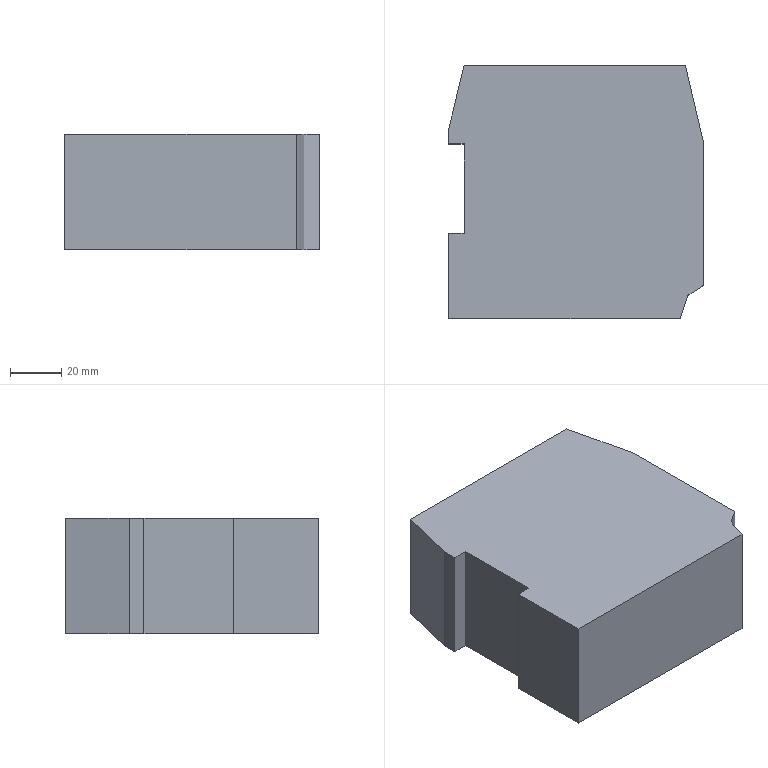Part | STEP file | EMC filter FIL-1S-1-10A-230AC-UT   1292320 | 1 solid | 14 faces | box 99.5 x 99 x 45 mm | volume 422145 mm3 | plane 14
STEP:
#1=CARTESIAN_POINT('',(0.,0.,0.));
#2=DIRECTION('',(0.,0.,1.));
#3=DIRECTION('',(1.,0.,0.));
#4=AXIS2_PLACEMENT_3D('',#1,#2,#3);
#5=CARTESIAN_POINT('',(49.75,18.24,0.));
#6=VERTEX_POINT('',#5);
#7=CARTESIAN_POINT('',(42.75,48.24,0.));
#8=VERTEX_POINT('',#7);
#9=CARTESIAN_POINT('',(42.75,48.24,0.));
#10=DIRECTION('',(-0.2272,0.9738,0.));
#11=VECTOR('',#10,1.);
#12=LINE('',#9,#11);
#13=CARTESIAN_POINT('',(42.75,48.24,45.));
#14=DIRECTION('',(-0.9738,-0.2272,0.));
#15=DIRECTION('',(0.2272,-0.9738,0.));
#16=AXIS2_PLACEMENT_3D('',#13,#14,#15);
#17=PLANE('',#16);
#18=CARTESIAN_POINT('',(0.,-45.));
#19=DIRECTION('',(-1.,0.));
#20=VECTOR('',#19,1.);
#21=LINE('',#18,#20);
#22=(GEOMETRIC_REPRESENTATION_CONTEXT(2)PARAMETRIC_REPRESENTATION_CONTEXT()REPRESENTATION_CONTEXT('',''));
#23=DEFINITIONAL_REPRESENTATION('',(#21),#22);
#24=PCURVE('',#17,#23);
#25=CARTESIAN_POINT('',(0.,0.,0.));
#26=DIRECTION('',(0.,0.,1.));
#27=DIRECTION('',(1.,0.,0.));
#28=AXIS2_PLACEMENT_3D('',#25,#26,#27);
#29=PLANE('',#28);
#30=CARTESIAN_POINT('',(42.75,48.24));
#31=DIRECTION('',(-0.2272,0.9738));
#32=VECTOR('',#31,1.);
#33=LINE('',#30,#32);
#34=(GEOMETRIC_REPRESENTATION_CONTEXT(2)PARAMETRIC_REPRESENTATION_CONTEXT()REPRESENTATION_CONTEXT('',''));
#35=DEFINITIONAL_REPRESENTATION('',(#33),#34);
#36=PCURVE('',#29,#35);
#37=SURFACE_CURVE('',#12,(#24,#36),.PCURVE_S1.);
#38=EDGE_CURVE('',#6,#8,#37,.T.);
#39=ORIENTED_EDGE('',*,*,#38,.T.);
#40=CARTESIAN_POINT('',(42.75,48.24,45.));
#41=VERTEX_POINT('',#40);
#42=CARTESIAN_POINT('',(42.75,48.24,45.));
#43=DIRECTION('',(0.,0.,-1.));
#44=VECTOR('',#43,1.);
#45=LINE('',#42,#44);
#46=CARTESIAN_POINT('',(0.,0.));
#47=DIRECTION('',(0.,-1.));
#48=VECTOR('',#47,1.);
#49=LINE('',#46,#48);
#50=(GEOMETRIC_REPRESENTATION_CONTEXT(2)PARAMETRIC_REPRESENTATION_CONTEXT()REPRESENTATION_CONTEXT('',''));
#51=DEFINITIONAL_REPRESENTATION('',(#49),#50);
#52=PCURVE('',#17,#51);
#53=CARTESIAN_POINT('',(-43.75,48.24,45.));
#54=DIRECTION('',(0.,-1.,0.));
#55=DIRECTION('',(0.,0.,-1.));
#56=AXIS2_PLACEMENT_3D('',#53,#54,#55);
#57=PLANE('',#56);
#58=CARTESIAN_POINT('',(0.,86.5));
#59=DIRECTION('',(1.,0.));
#60=VECTOR('',#59,1.);
#61=LINE('',#58,#60);
#62=(GEOMETRIC_REPRESENTATION_CONTEXT(2)PARAMETRIC_REPRESENTATION_CONTEXT()REPRESENTATION_CONTEXT('',''));
#63=DEFINITIONAL_REPRESENTATION('',(#61),#62);
#64=PCURVE('',#57,#63);
#65=SURFACE_CURVE('',#45,(#52,#64),.PCURVE_S1.);
#66=EDGE_CURVE('',#41,#8,#65,.T.);
#67=ORIENTED_EDGE('',*,*,#66,.F.);
#68=CARTESIAN_POINT('',(49.75,18.24,45.));
#69=VERTEX_POINT('',#68);
#70=CARTESIAN_POINT('',(42.75,48.24,45.));
#71=DIRECTION('',(-0.2272,0.9738,0.));
#72=VECTOR('',#71,1.);
#73=LINE('',#70,#72);
#74=CARTESIAN_POINT('',(0.,0.));
#75=DIRECTION('',(-1.,0.));
#76=VECTOR('',#75,1.);
#77=LINE('',#74,#76);
#78=(GEOMETRIC_REPRESENTATION_CONTEXT(2)PARAMETRIC_REPRESENTATION_CONTEXT()REPRESENTATION_CONTEXT('',''));
#79=DEFINITIONAL_REPRESENTATION('',(#77),#78);
#80=PCURVE('',#17,#79);
#81=CARTESIAN_POINT('',(0.,0.,45.));
#82=DIRECTION('',(0.,0.,1.));
#83=DIRECTION('',(1.,0.,0.));
#84=AXIS2_PLACEMENT_3D('',#81,#82,#83);
#85=PLANE('',#84);
#86=CARTESIAN_POINT('',(42.75,48.24));
#87=DIRECTION('',(-0.2272,0.9738));
#88=VECTOR('',#87,1.);
#89=LINE('',#86,#88);
#90=(GEOMETRIC_REPRESENTATION_CONTEXT(2)PARAMETRIC_REPRESENTATION_CONTEXT()REPRESENTATION_CONTEXT('',''));
#91=DEFINITIONAL_REPRESENTATION('',(#89),#90);
#92=PCURVE('',#85,#91);
#93=SURFACE_CURVE('',#73,(#80,#92),.PCURVE_S1.);
#94=EDGE_CURVE('',#69,#41,#93,.T.);
#95=ORIENTED_EDGE('',*,*,#94,.F.);
#96=CARTESIAN_POINT('',(49.75,18.24,45.));
#97=DIRECTION('',(0.,0.,-1.));
#98=VECTOR('',#97,1.);
#99=LINE('',#96,#98);
#100=CARTESIAN_POINT('',(30.806,0.));
#101=DIRECTION('',(0.,-1.));
#102=VECTOR('',#101,1.);
#103=LINE('',#100,#102);
#104=(GEOMETRIC_REPRESENTATION_CONTEXT(2)PARAMETRIC_REPRESENTATION_CONTEXT()REPRESENTATION_CONTEXT('',''));
#105=DEFINITIONAL_REPRESENTATION('',(#103),#104);
#106=PCURVE('',#17,#105);
#107=CARTESIAN_POINT('',(49.75,18.24,45.));
#108=DIRECTION('',(-1.,0.,0.));
#109=DIRECTION('',(0.,-1.,0.));
#110=AXIS2_PLACEMENT_3D('',#107,#108,#109);
#111=PLANE('',#110);
#112=CARTESIAN_POINT('',(0.,0.));
#113=DIRECTION('',(0.,-1.));
#114=VECTOR('',#113,1.);
#115=LINE('',#112,#114);
#116=(GEOMETRIC_REPRESENTATION_CONTEXT(2)PARAMETRIC_REPRESENTATION_CONTEXT()REPRESENTATION_CONTEXT('',''));
#117=DEFINITIONAL_REPRESENTATION('',(#115),#116);
#118=PCURVE('',#111,#117);
#119=SURFACE_CURVE('',#99,(#106,#118),.PCURVE_S1.);
#120=EDGE_CURVE('',#69,#6,#119,.T.);
#121=ORIENTED_EDGE('',*,*,#120,.T.);
#122=EDGE_LOOP('',(#39,#67,#95,#121));
#123=FACE_BOUND('',#122,.T.);
#124=ADVANCED_FACE('',(#123),#17,.F.);
#125=CARTESIAN_POINT('',(-43.75,48.24,0.));
#126=VERTEX_POINT('',#125);
#127=CARTESIAN_POINT('',(-43.75,48.24,0.));
#128=DIRECTION('',(-1.,0.,0.));
#129=VECTOR('',#128,1.);
#130=LINE('',#127,#129);
#131=CARTESIAN_POINT('',(45.,0.));
#132=DIRECTION('',(0.,-1.));
#133=VECTOR('',#132,1.);
#134=LINE('',#131,#133);
#135=(GEOMETRIC_REPRESENTATION_CONTEXT(2)PARAMETRIC_REPRESENTATION_CONTEXT()REPRESENTATION_CONTEXT('',''));
#136=DEFINITIONAL_REPRESENTATION('',(#134),#135);
#137=PCURVE('',#57,#136);
#138=CARTESIAN_POINT('',(-43.75,48.24));
#139=DIRECTION('',(-1.,0.));
#140=VECTOR('',#139,1.);
#141=LINE('',#138,#140);
#142=(GEOMETRIC_REPRESENTATION_CONTEXT(2)PARAMETRIC_REPRESENTATION_CONTEXT()REPRESENTATION_CONTEXT('',''));
#143=DEFINITIONAL_REPRESENTATION('',(#141),#142);
#144=PCURVE('',#29,#143);
#145=SURFACE_CURVE('',#130,(#137,#144),.PCURVE_S1.);
#146=EDGE_CURVE('',#8,#126,#145,.T.);
#147=ORIENTED_EDGE('',*,*,#146,.T.);
#148=CARTESIAN_POINT('',(-43.75,48.24,45.));
#149=VERTEX_POINT('',#148);
#150=CARTESIAN_POINT('',(-43.75,48.24,45.));
#151=DIRECTION('',(0.,0.,-1.));
#152=VECTOR('',#151,1.);
#153=LINE('',#150,#152);
#154=CARTESIAN_POINT('',(0.,0.));
#155=DIRECTION('',(1.,0.));
#156=VECTOR('',#155,1.);
#157=LINE('',#154,#156);
#158=(GEOMETRIC_REPRESENTATION_CONTEXT(2)PARAMETRIC_REPRESENTATION_CONTEXT()REPRESENTATION_CONTEXT('',''));
#159=DEFINITIONAL_REPRESENTATION('',(#157),#158);
#160=PCURVE('',#57,#159);
#161=CARTESIAN_POINT('',(-49.75,23.24,45.));
#162=DIRECTION('',(0.9724,-0.2334,0.));
#163=DIRECTION('',(0.2334,0.9724,0.));
#164=AXIS2_PLACEMENT_3D('',#161,#162,#163);
#165=PLANE('',#164);
#166=CARTESIAN_POINT('',(25.71,0.));
#167=DIRECTION('',(0.,-1.));
#168=VECTOR('',#167,1.);
#169=LINE('',#166,#168);
#170=(GEOMETRIC_REPRESENTATION_CONTEXT(2)PARAMETRIC_REPRESENTATION_CONTEXT()REPRESENTATION_CONTEXT('',''));
#171=DEFINITIONAL_REPRESENTATION('',(#169),#170);
#172=PCURVE('',#165,#171);
#173=SURFACE_CURVE('',#153,(#160,#172),.PCURVE_S1.);
#174=EDGE_CURVE('',#149,#126,#173,.T.);
#175=ORIENTED_EDGE('',*,*,#174,.F.);
#176=CARTESIAN_POINT('',(-43.75,48.24,45.));
#177=DIRECTION('',(-1.,0.,0.));
#178=VECTOR('',#177,1.);
#179=LINE('',#176,#178);
#180=CARTESIAN_POINT('',(0.,0.));
#181=DIRECTION('',(0.,-1.));
#182=VECTOR('',#181,1.);
#183=LINE('',#180,#182);
#184=(GEOMETRIC_REPRESENTATION_CONTEXT(2)PARAMETRIC_REPRESENTATION_CONTEXT()REPRESENTATION_CONTEXT('',''));
#185=DEFINITIONAL_REPRESENTATION('',(#183),#184);
#186=PCURVE('',#57,#185);
#187=CARTESIAN_POINT('',(-43.75,48.24));
#188=DIRECTION('',(-1.,0.));
#189=VECTOR('',#188,1.);
#190=LINE('',#187,#189);
#191=(GEOMETRIC_REPRESENTATION_CONTEXT(2)PARAMETRIC_REPRESENTATION_CONTEXT()REPRESENTATION_CONTEXT('',''));
#192=DEFINITIONAL_REPRESENTATION('',(#190),#191);
#193=PCURVE('',#85,#192);
#194=SURFACE_CURVE('',#179,(#186,#193),.PCURVE_S1.);
#195=EDGE_CURVE('',#41,#149,#194,.T.);
#196=ORIENTED_EDGE('',*,*,#195,.F.);
#197=ORIENTED_EDGE('',*,*,#66,.T.);
#198=EDGE_LOOP('',(#147,#175,#196,#197));
#199=FACE_BOUND('',#198,.T.);
#200=ADVANCED_FACE('',(#199),#57,.F.);
#201=CARTESIAN_POINT('',(-49.75,23.24,0.));
#202=VERTEX_POINT('',#201);
#203=CARTESIAN_POINT('',(-49.75,23.24,0.));
#204=DIRECTION('',(-0.2334,-0.9724,0.));
#205=VECTOR('',#204,1.);
#206=LINE('',#203,#205);
#207=CARTESIAN_POINT('',(0.,-45.));
#208=DIRECTION('',(-1.,0.));
#209=VECTOR('',#208,1.);
#210=LINE('',#207,#209);
#211=(GEOMETRIC_REPRESENTATION_CONTEXT(2)PARAMETRIC_REPRESENTATION_CONTEXT()REPRESENTATION_CONTEXT('',''));
#212=DEFINITIONAL_REPRESENTATION('',(#210),#211);
#213=PCURVE('',#165,#212);
#214=CARTESIAN_POINT('',(-49.75,23.24));
#215=DIRECTION('',(-0.2334,-0.9724));
#216=VECTOR('',#215,1.);
#217=LINE('',#214,#216);
#218=(GEOMETRIC_REPRESENTATION_CONTEXT(2)PARAMETRIC_REPRESENTATION_CONTEXT()REPRESENTATION_CONTEXT('',''));
#219=DEFINITIONAL_REPRESENTATION('',(#217),#218);
#220=PCURVE('',#29,#219);
#221=SURFACE_CURVE('',#206,(#213,#220),.PCURVE_S1.);
#222=EDGE_CURVE('',#126,#202,#221,.T.);
#223=ORIENTED_EDGE('',*,*,#222,.T.);
#224=CARTESIAN_POINT('',(-49.75,23.24,45.));
#225=VERTEX_POINT('',#224);
#226=CARTESIAN_POINT('',(-49.75,23.24,45.));
#227=DIRECTION('',(0.,0.,-1.));
#228=VECTOR('',#227,1.);
#229=LINE('',#226,#228);
#230=CARTESIAN_POINT('',(0.,0.));
#231=DIRECTION('',(0.,-1.));
#232=VECTOR('',#231,1.);
#233=LINE('',#230,#232);
#234=(GEOMETRIC_REPRESENTATION_CONTEXT(2)PARAMETRIC_REPRESENTATION_CONTEXT()REPRESENTATION_CONTEXT('',''));
#235=DEFINITIONAL_REPRESENTATION('',(#233),#234);
#236=PCURVE('',#165,#235);
#237=CARTESIAN_POINT('',(-49.75,23.24,45.));
#238=DIRECTION('',(1.,0.,0.));
#239=DIRECTION('',(0.,0.,-1.));
#240=AXIS2_PLACEMENT_3D('',#237,#238,#239);
#241=PLANE('',#240);
#242=CARTESIAN_POINT('',(0.,0.));
#243=DIRECTION('',(1.,0.));
#244=VECTOR('',#243,1.);
#245=LINE('',#242,#244);
#246=(GEOMETRIC_REPRESENTATION_CONTEXT(2)PARAMETRIC_REPRESENTATION_CONTEXT()REPRESENTATION_CONTEXT('',''));
#247=DEFINITIONAL_REPRESENTATION('',(#245),#246);
#248=PCURVE('',#241,#247);
#249=SURFACE_CURVE('',#229,(#236,#248),.PCURVE_S1.);
#250=EDGE_CURVE('',#225,#202,#249,.T.);
#251=ORIENTED_EDGE('',*,*,#250,.F.);
#252=CARTESIAN_POINT('',(-49.75,23.24,45.));
#253=DIRECTION('',(-0.2334,-0.9724,0.));
#254=VECTOR('',#253,1.);
#255=LINE('',#252,#254);
#256=CARTESIAN_POINT('',(0.,0.));
#257=DIRECTION('',(-1.,0.));
#258=VECTOR('',#257,1.);
#259=LINE('',#256,#258);
#260=(GEOMETRIC_REPRESENTATION_CONTEXT(2)PARAMETRIC_REPRESENTATION_CONTEXT()REPRESENTATION_CONTEXT('',''));
#261=DEFINITIONAL_REPRESENTATION('',(#259),#260);
#262=PCURVE('',#165,#261);
#263=CARTESIAN_POINT('',(-49.75,23.24));
#264=DIRECTION('',(-0.2334,-0.9724));
#265=VECTOR('',#264,1.);
#266=LINE('',#263,#265);
#267=(GEOMETRIC_REPRESENTATION_CONTEXT(2)PARAMETRIC_REPRESENTATION_CONTEXT()REPRESENTATION_CONTEXT('',''));
#268=DEFINITIONAL_REPRESENTATION('',(#266),#267);
#269=PCURVE('',#85,#268);
#270=SURFACE_CURVE('',#255,(#262,#269),.PCURVE_S1.);
#271=EDGE_CURVE('',#149,#225,#270,.T.);
#272=ORIENTED_EDGE('',*,*,#271,.F.);
#273=ORIENTED_EDGE('',*,*,#174,.T.);
#274=EDGE_LOOP('',(#223,#251,#272,#273));
#275=FACE_BOUND('',#274,.T.);
#276=ADVANCED_FACE('',(#275),#165,.F.);
#277=CARTESIAN_POINT('',(-49.75,17.5,0.));
#278=VERTEX_POINT('',#277);
#279=CARTESIAN_POINT('',(-49.75,23.24,0.));
#280=DIRECTION('',(0.,-1.,0.));
#281=VECTOR('',#280,1.);
#282=LINE('',#279,#281);
#283=CARTESIAN_POINT('',(45.,0.));
#284=DIRECTION('',(0.,-1.));
#285=VECTOR('',#284,1.);
#286=LINE('',#283,#285);
#287=(GEOMETRIC_REPRESENTATION_CONTEXT(2)PARAMETRIC_REPRESENTATION_CONTEXT()REPRESENTATION_CONTEXT('',''));
#288=DEFINITIONAL_REPRESENTATION('',(#286),#287);
#289=PCURVE('',#241,#288);
#290=CARTESIAN_POINT('',(-49.75,23.24));
#291=DIRECTION('',(0.,-1.));
#292=VECTOR('',#291,1.);
#293=LINE('',#290,#292);
#294=(GEOMETRIC_REPRESENTATION_CONTEXT(2)PARAMETRIC_REPRESENTATION_CONTEXT()REPRESENTATION_CONTEXT('',''));
#295=DEFINITIONAL_REPRESENTATION('',(#293),#294);
#296=PCURVE('',#29,#295);
#297=SURFACE_CURVE('',#282,(#289,#296),.PCURVE_S1.);
#298=EDGE_CURVE('',#202,#278,#297,.T.);
#299=ORIENTED_EDGE('',*,*,#298,.T.);
#300=CARTESIAN_POINT('',(-49.75,17.5,45.));
#301=VERTEX_POINT('',#300);
#302=CARTESIAN_POINT('',(-49.75,17.5,45.));
#303=DIRECTION('',(0.,0.,-1.));
#304=VECTOR('',#303,1.);
#305=LINE('',#302,#304);
#306=CARTESIAN_POINT('',(0.,-5.74));
#307=DIRECTION('',(1.,0.));
#308=VECTOR('',#307,1.);
#309=LINE('',#306,#308);
#310=(GEOMETRIC_REPRESENTATION_CONTEXT(2)PARAMETRIC_REPRESENTATION_CONTEXT()REPRESENTATION_CONTEXT('',''));
#311=DEFINITIONAL_REPRESENTATION('',(#309),#310);
#312=PCURVE('',#241,#311);
#313=CARTESIAN_POINT('',(-49.75,17.5,45.));
#314=DIRECTION('',(0.,1.,0.));
#315=DIRECTION('',(0.,0.,1.));
#316=AXIS2_PLACEMENT_3D('',#313,#314,#315);
#317=PLANE('',#316);
#318=CARTESIAN_POINT('',(0.,0.));
#319=DIRECTION('',(-1.,0.));
#320=VECTOR('',#319,1.);
#321=LINE('',#318,#320);
#322=(GEOMETRIC_REPRESENTATION_CONTEXT(2)PARAMETRIC_REPRESENTATION_CONTEXT()REPRESENTATION_CONTEXT('',''));
#323=DEFINITIONAL_REPRESENTATION('',(#321),#322);
#324=PCURVE('',#317,#323);
#325=SURFACE_CURVE('',#305,(#312,#324),.PCURVE_S1.);
#326=EDGE_CURVE('',#301,#278,#325,.T.);
#327=ORIENTED_EDGE('',*,*,#326,.F.);
#328=CARTESIAN_POINT('',(-49.75,23.24,45.));
#329=DIRECTION('',(0.,-1.,0.));
#330=VECTOR('',#329,1.);
#331=LINE('',#328,#330);
#332=CARTESIAN_POINT('',(0.,0.));
#333=DIRECTION('',(0.,-1.));
#334=VECTOR('',#333,1.);
#335=LINE('',#332,#334);
#336=(GEOMETRIC_REPRESENTATION_CONTEXT(2)PARAMETRIC_REPRESENTATION_CONTEXT()REPRESENTATION_CONTEXT('',''));
#337=DEFINITIONAL_REPRESENTATION('',(#335),#336);
#338=PCURVE('',#241,#337);
#339=CARTESIAN_POINT('',(-49.75,23.24));
#340=DIRECTION('',(0.,-1.));
#341=VECTOR('',#340,1.);
#342=LINE('',#339,#341);
#343=(GEOMETRIC_REPRESENTATION_CONTEXT(2)PARAMETRIC_REPRESENTATION_CONTEXT()REPRESENTATION_CONTEXT('',''));
#344=DEFINITIONAL_REPRESENTATION('',(#342),#343);
#345=PCURVE('',#85,#344);
#346=SURFACE_CURVE('',#331,(#338,#345),.PCURVE_S1.);
#347=EDGE_CURVE('',#225,#301,#346,.T.);
#348=ORIENTED_EDGE('',*,*,#347,.F.);
#349=ORIENTED_EDGE('',*,*,#250,.T.);
#350=EDGE_LOOP('',(#299,#327,#348,#349));
#351=FACE_BOUND('',#350,.T.);
#352=ADVANCED_FACE('',(#351),#241,.F.);
#353=CARTESIAN_POINT('',(-43.75,17.5,0.));
#354=VERTEX_POINT('',#353);
#355=CARTESIAN_POINT('',(-49.75,17.5,0.));
#356=DIRECTION('',(1.,0.,0.));
#357=VECTOR('',#356,1.);
#358=LINE('',#355,#357);
#359=CARTESIAN_POINT('',(-45.,0.));
#360=DIRECTION('',(0.,1.));
#361=VECTOR('',#360,1.);
#362=LINE('',#359,#361);
#363=(GEOMETRIC_REPRESENTATION_CONTEXT(2)PARAMETRIC_REPRESENTATION_CONTEXT()REPRESENTATION_CONTEXT('',''));
#364=DEFINITIONAL_REPRESENTATION('',(#362),#363);
#365=PCURVE('',#317,#364);
#366=CARTESIAN_POINT('',(-49.75,17.5));
#367=DIRECTION('',(1.,0.));
#368=VECTOR('',#367,1.);
#369=LINE('',#366,#368);
#370=(GEOMETRIC_REPRESENTATION_CONTEXT(2)PARAMETRIC_REPRESENTATION_CONTEXT()REPRESENTATION_CONTEXT('',''));
#371=DEFINITIONAL_REPRESENTATION('',(#369),#370);
#372=PCURVE('',#29,#371);
#373=SURFACE_CURVE('',#358,(#365,#372),.PCURVE_S1.);
#374=EDGE_CURVE('',#278,#354,#373,.T.);
#375=ORIENTED_EDGE('',*,*,#374,.T.);
#376=CARTESIAN_POINT('',(-43.75,17.5,45.));
#377=VERTEX_POINT('',#376);
#378=CARTESIAN_POINT('',(-43.75,17.5,45.));
#379=DIRECTION('',(0.,0.,-1.));
#380=VECTOR('',#379,1.);
#381=LINE('',#378,#380);
#382=CARTESIAN_POINT('',(0.,6.));
#383=DIRECTION('',(-1.,0.));
#384=VECTOR('',#383,1.);
#385=LINE('',#382,#384);
#386=(GEOMETRIC_REPRESENTATION_CONTEXT(2)PARAMETRIC_REPRESENTATION_CONTEXT()REPRESENTATION_CONTEXT('',''));
#387=DEFINITIONAL_REPRESENTATION('',(#385),#386);
#388=PCURVE('',#317,#387);
#389=CARTESIAN_POINT('',(-43.75,17.5,45.));
#390=DIRECTION('',(1.,0.,0.));
#391=DIRECTION('',(0.,0.,-1.));
#392=AXIS2_PLACEMENT_3D('',#389,#390,#391);
#393=PLANE('',#392);
#394=CARTESIAN_POINT('',(0.,0.));
#395=DIRECTION('',(1.,0.));
#396=VECTOR('',#395,1.);
#397=LINE('',#394,#396);
#398=(GEOMETRIC_REPRESENTATION_CONTEXT(2)PARAMETRIC_REPRESENTATION_CONTEXT()REPRESENTATION_CONTEXT('',''));
#399=DEFINITIONAL_REPRESENTATION('',(#397),#398);
#400=PCURVE('',#393,#399);
#401=SURFACE_CURVE('',#381,(#388,#400),.PCURVE_S1.);
#402=EDGE_CURVE('',#377,#354,#401,.T.);
#403=ORIENTED_EDGE('',*,*,#402,.F.);
#404=CARTESIAN_POINT('',(-49.75,17.5,45.));
#405=DIRECTION('',(1.,0.,0.));
#406=VECTOR('',#405,1.);
#407=LINE('',#404,#406);
#408=CARTESIAN_POINT('',(0.,0.));
#409=DIRECTION('',(0.,1.));
#410=VECTOR('',#409,1.);
#411=LINE('',#408,#410);
#412=(GEOMETRIC_REPRESENTATION_CONTEXT(2)PARAMETRIC_REPRESENTATION_CONTEXT()REPRESENTATION_CONTEXT('',''));
#413=DEFINITIONAL_REPRESENTATION('',(#411),#412);
#414=PCURVE('',#317,#413);
#415=CARTESIAN_POINT('',(-49.75,17.5));
#416=DIRECTION('',(1.,0.));
#417=VECTOR('',#416,1.);
#418=LINE('',#415,#417);
#419=(GEOMETRIC_REPRESENTATION_CONTEXT(2)PARAMETRIC_REPRESENTATION_CONTEXT()REPRESENTATION_CONTEXT('',''));
#420=DEFINITIONAL_REPRESENTATION('',(#418),#419);
#421=PCURVE('',#85,#420);
#422=SURFACE_CURVE('',#407,(#414,#421),.PCURVE_S1.);
#423=EDGE_CURVE('',#301,#377,#422,.T.);
#424=ORIENTED_EDGE('',*,*,#423,.F.);
#425=ORIENTED_EDGE('',*,*,#326,.T.);
#426=EDGE_LOOP('',(#375,#403,#424,#425));
#427=FACE_BOUND('',#426,.T.);
#428=ADVANCED_FACE('',(#427),#317,.F.);
#429=CARTESIAN_POINT('',(-43.75,-17.5,0.));
#430=VERTEX_POINT('',#429);
#431=CARTESIAN_POINT('',(-43.75,17.5,0.));
#432=DIRECTION('',(0.,-1.,0.));
#433=VECTOR('',#432,1.);
#434=LINE('',#431,#433);
#435=CARTESIAN_POINT('',(45.,0.));
#436=DIRECTION('',(0.,-1.));
#437=VECTOR('',#436,1.);
#438=LINE('',#435,#437);
#439=(GEOMETRIC_REPRESENTATION_CONTEXT(2)PARAMETRIC_REPRESENTATION_CONTEXT()REPRESENTATION_CONTEXT('',''));
#440=DEFINITIONAL_REPRESENTATION('',(#438),#439);
#441=PCURVE('',#393,#440);
#442=CARTESIAN_POINT('',(-43.75,17.5));
#443=DIRECTION('',(0.,-1.));
#444=VECTOR('',#443,1.);
#445=LINE('',#442,#444);
#446=(GEOMETRIC_REPRESENTATION_CONTEXT(2)PARAMETRIC_REPRESENTATION_CONTEXT()REPRESENTATION_CONTEXT('',''));
#447=DEFINITIONAL_REPRESENTATION('',(#445),#446);
#448=PCURVE('',#29,#447);
#449=SURFACE_CURVE('',#434,(#441,#448),.PCURVE_S1.);
#450=EDGE_CURVE('',#354,#430,#449,.T.);
#451=ORIENTED_EDGE('',*,*,#450,.T.);
#452=CARTESIAN_POINT('',(-43.75,-17.5,45.));
#453=VERTEX_POINT('',#452);
#454=CARTESIAN_POINT('',(-43.75,-17.5,45.));
#455=DIRECTION('',(0.,0.,-1.));
#456=VECTOR('',#455,1.);
#457=LINE('',#454,#456);
#458=CARTESIAN_POINT('',(0.,-35.));
#459=DIRECTION('',(1.,0.));
#460=VECTOR('',#459,1.);
#461=LINE('',#458,#460);
#462=(GEOMETRIC_REPRESENTATION_CONTEXT(2)PARAMETRIC_REPRESENTATION_CONTEXT()REPRESENTATION_CONTEXT('',''));
#463=DEFINITIONAL_REPRESENTATION('',(#461),#462);
#464=PCURVE('',#393,#463);
#465=CARTESIAN_POINT('',(-49.75,-17.5,45.));
#466=DIRECTION('',(0.,-1.,0.));
#467=DIRECTION('',(0.,0.,-1.));
#468=AXIS2_PLACEMENT_3D('',#465,#466,#467);
#469=PLANE('',#468);
#470=CARTESIAN_POINT('',(0.,6.));
#471=DIRECTION('',(1.,0.));
#472=VECTOR('',#471,1.);
#473=LINE('',#470,#472);
#474=(GEOMETRIC_REPRESENTATION_CONTEXT(2)PARAMETRIC_REPRESENTATION_CONTEXT()REPRESENTATION_CONTEXT('',''));
#475=DEFINITIONAL_REPRESENTATION('',(#473),#474);
#476=PCURVE('',#469,#475);
#477=SURFACE_CURVE('',#457,(#464,#476),.PCURVE_S1.);
#478=EDGE_CURVE('',#453,#430,#477,.T.);
#479=ORIENTED_EDGE('',*,*,#478,.F.);
#480=CARTESIAN_POINT('',(-43.75,17.5,45.));
#481=DIRECTION('',(0.,-1.,0.));
#482=VECTOR('',#481,1.);
#483=LINE('',#480,#482);
#484=CARTESIAN_POINT('',(0.,0.));
#485=DIRECTION('',(0.,-1.));
#486=VECTOR('',#485,1.);
#487=LINE('',#484,#486);
#488=(GEOMETRIC_REPRESENTATION_CONTEXT(2)PARAMETRIC_REPRESENTATION_CONTEXT()REPRESENTATION_CONTEXT('',''));
#489=DEFINITIONAL_REPRESENTATION('',(#487),#488);
#490=PCURVE('',#393,#489);
#491=CARTESIAN_POINT('',(-43.75,17.5));
#492=DIRECTION('',(0.,-1.));
#493=VECTOR('',#492,1.);
#494=LINE('',#491,#493);
#495=(GEOMETRIC_REPRESENTATION_CONTEXT(2)PARAMETRIC_REPRESENTATION_CONTEXT()REPRESENTATION_CONTEXT('',''));
#496=DEFINITIONAL_REPRESENTATION('',(#494),#495);
#497=PCURVE('',#85,#496);
#498=SURFACE_CURVE('',#483,(#490,#497),.PCURVE_S1.);
#499=EDGE_CURVE('',#377,#453,#498,.T.);
#500=ORIENTED_EDGE('',*,*,#499,.F.);
#501=ORIENTED_EDGE('',*,*,#402,.T.);
#502=EDGE_LOOP('',(#451,#479,#500,#501));
#503=FACE_BOUND('',#502,.T.);
#504=ADVANCED_FACE('',(#503),#393,.F.);
#505=CARTESIAN_POINT('',(-49.75,-17.5,0.));
#506=VERTEX_POINT('',#505);
#507=CARTESIAN_POINT('',(-49.75,-17.5,0.));
#508=DIRECTION('',(-1.,0.,0.));
#509=VECTOR('',#508,1.);
#510=LINE('',#507,#509);
#511=CARTESIAN_POINT('',(45.,0.));
#512=DIRECTION('',(0.,-1.));
#513=VECTOR('',#512,1.);
#514=LINE('',#511,#513);
#515=(GEOMETRIC_REPRESENTATION_CONTEXT(2)PARAMETRIC_REPRESENTATION_CONTEXT()REPRESENTATION_CONTEXT('',''));
#516=DEFINITIONAL_REPRESENTATION('',(#514),#515);
#517=PCURVE('',#469,#516);
#518=CARTESIAN_POINT('',(-49.75,-17.5));
#519=DIRECTION('',(-1.,0.));
#520=VECTOR('',#519,1.);
#521=LINE('',#518,#520);
#522=(GEOMETRIC_REPRESENTATION_CONTEXT(2)PARAMETRIC_REPRESENTATION_CONTEXT()REPRESENTATION_CONTEXT('',''));
#523=DEFINITIONAL_REPRESENTATION('',(#521),#522);
#524=PCURVE('',#29,#523);
#525=SURFACE_CURVE('',#510,(#517,#524),.PCURVE_S1.);
#526=EDGE_CURVE('',#430,#506,#525,.T.);
#527=ORIENTED_EDGE('',*,*,#526,.T.);
#528=CARTESIAN_POINT('',(-49.75,-17.5,45.));
#529=VERTEX_POINT('',#528);
#530=CARTESIAN_POINT('',(-49.75,-17.5,45.));
#531=DIRECTION('',(0.,0.,-1.));
#532=VECTOR('',#531,1.);
#533=LINE('',#530,#532);
#534=CARTESIAN_POINT('',(0.,0.));
#535=DIRECTION('',(1.,0.));
#536=VECTOR('',#535,1.);
#537=LINE('',#534,#536);
#538=(GEOMETRIC_REPRESENTATION_CONTEXT(2)PARAMETRIC_REPRESENTATION_CONTEXT()REPRESENTATION_CONTEXT('',''));
#539=DEFINITIONAL_REPRESENTATION('',(#537),#538);
#540=PCURVE('',#469,#539);
#541=CARTESIAN_POINT('',(-49.75,-17.5,45.));
#542=DIRECTION('',(1.,0.,0.));
#543=DIRECTION('',(0.,1.,0.));
#544=AXIS2_PLACEMENT_3D('',#541,#542,#543);
#545=PLANE('',#544);
#546=CARTESIAN_POINT('',(0.,0.));
#547=DIRECTION('',(0.,-1.));
#548=VECTOR('',#547,1.);
#549=LINE('',#546,#548);
#550=(GEOMETRIC_REPRESENTATION_CONTEXT(2)PARAMETRIC_REPRESENTATION_CONTEXT()REPRESENTATION_CONTEXT('',''));
#551=DEFINITIONAL_REPRESENTATION('',(#549),#550);
#552=PCURVE('',#545,#551);
#553=SURFACE_CURVE('',#533,(#540,#552),.PCURVE_S1.);
#554=EDGE_CURVE('',#529,#506,#553,.T.);
#555=ORIENTED_EDGE('',*,*,#554,.F.);
#556=CARTESIAN_POINT('',(-49.75,-17.5,45.));
#557=DIRECTION('',(-1.,0.,0.));
#558=VECTOR('',#557,1.);
#559=LINE('',#556,#558);
#560=CARTESIAN_POINT('',(0.,0.));
#561=DIRECTION('',(0.,-1.));
#562=VECTOR('',#561,1.);
#563=LINE('',#560,#562);
#564=(GEOMETRIC_REPRESENTATION_CONTEXT(2)PARAMETRIC_REPRESENTATION_CONTEXT()REPRESENTATION_CONTEXT('',''));
#565=DEFINITIONAL_REPRESENTATION('',(#563),#564);
#566=PCURVE('',#469,#565);
#567=CARTESIAN_POINT('',(-49.75,-17.5));
#568=DIRECTION('',(-1.,0.));
#569=VECTOR('',#568,1.);
#570=LINE('',#567,#569);
#571=(GEOMETRIC_REPRESENTATION_CONTEXT(2)PARAMETRIC_REPRESENTATION_CONTEXT()REPRESENTATION_CONTEXT('',''));
#572=DEFINITIONAL_REPRESENTATION('',(#570),#571);
#573=PCURVE('',#85,#572);
#574=SURFACE_CURVE('',#559,(#566,#573),.PCURVE_S1.);
#575=EDGE_CURVE('',#453,#529,#574,.T.);
#576=ORIENTED_EDGE('',*,*,#575,.F.);
#577=ORIENTED_EDGE('',*,*,#478,.T.);
#578=EDGE_LOOP('',(#527,#555,#576,#577));
#579=FACE_BOUND('',#578,.T.);
#580=ADVANCED_FACE('',(#579),#469,.F.);
#581=CARTESIAN_POINT('',(-49.75,-50.76,0.));
#582=VERTEX_POINT('',#581);
#583=CARTESIAN_POINT('',(-49.75,-17.5,0.));
#584=DIRECTION('',(0.,-1.,0.));
#585=VECTOR('',#584,1.);
#586=LINE('',#583,#585);
#587=CARTESIAN_POINT('',(0.,-45.));
#588=DIRECTION('',(-1.,0.));
#589=VECTOR('',#588,1.);
#590=LINE('',#587,#589);
#591=(GEOMETRIC_REPRESENTATION_CONTEXT(2)PARAMETRIC_REPRESENTATION_CONTEXT()REPRESENTATION_CONTEXT('',''));
#592=DEFINITIONAL_REPRESENTATION('',(#590),#591);
#593=PCURVE('',#545,#592);
#594=CARTESIAN_POINT('',(-49.75,-17.5));
#595=DIRECTION('',(0.,-1.));
#596=VECTOR('',#595,1.);
#597=LINE('',#594,#596);
#598=(GEOMETRIC_REPRESENTATION_CONTEXT(2)PARAMETRIC_REPRESENTATION_CONTEXT()REPRESENTATION_CONTEXT('',''));
#599=DEFINITIONAL_REPRESENTATION('',(#597),#598);
#600=PCURVE('',#29,#599);
#601=SURFACE_CURVE('',#586,(#593,#600),.PCURVE_S1.);
#602=EDGE_CURVE('',#506,#582,#601,.T.);
#603=ORIENTED_EDGE('',*,*,#602,.T.);
#604=CARTESIAN_POINT('',(-49.75,-50.76,45.));
#605=VERTEX_POINT('',#604);
#606=CARTESIAN_POINT('',(-49.75,-50.76,45.));
#607=DIRECTION('',(0.,0.,-1.));
#608=VECTOR('',#607,1.);
#609=LINE('',#606,#608);
#610=CARTESIAN_POINT('',(-33.26,0.));
#611=DIRECTION('',(0.,-1.));
#612=VECTOR('',#611,1.);
#613=LINE('',#610,#612);
#614=(GEOMETRIC_REPRESENTATION_CONTEXT(2)PARAMETRIC_REPRESENTATION_CONTEXT()REPRESENTATION_CONTEXT('',''));
#615=DEFINITIONAL_REPRESENTATION('',(#613),#614);
#616=PCURVE('',#545,#615);
#617=CARTESIAN_POINT('',(-49.75,-50.76,45.));
#618=DIRECTION('',(0.,1.,0.));
#619=DIRECTION('',(0.,0.,1.));
#620=AXIS2_PLACEMENT_3D('',#617,#618,#619);
#621=PLANE('',#620);
#622=CARTESIAN_POINT('',(0.,0.));
#623=DIRECTION('',(-1.,0.));
#624=VECTOR('',#623,1.);
#625=LINE('',#622,#624);
#626=(GEOMETRIC_REPRESENTATION_CONTEXT(2)PARAMETRIC_REPRESENTATION_CONTEXT()REPRESENTATION_CONTEXT('',''));
#627=DEFINITIONAL_REPRESENTATION('',(#625),#626);
#628=PCURVE('',#621,#627);
#629=SURFACE_CURVE('',#609,(#616,#628),.PCURVE_S1.);
#630=EDGE_CURVE('',#605,#582,#629,.T.);
#631=ORIENTED_EDGE('',*,*,#630,.F.);
#632=CARTESIAN_POINT('',(-49.75,-17.5,45.));
#633=DIRECTION('',(0.,-1.,0.));
#634=VECTOR('',#633,1.);
#635=LINE('',#632,#634);
#636=CARTESIAN_POINT('',(0.,0.));
#637=DIRECTION('',(-1.,0.));
#638=VECTOR('',#637,1.);
#639=LINE('',#636,#638);
#640=(GEOMETRIC_REPRESENTATION_CONTEXT(2)PARAMETRIC_REPRESENTATION_CONTEXT()REPRESENTATION_CONTEXT('',''));
#641=DEFINITIONAL_REPRESENTATION('',(#639),#640);
#642=PCURVE('',#545,#641);
#643=CARTESIAN_POINT('',(-49.75,-17.5));
#644=DIRECTION('',(0.,-1.));
#645=VECTOR('',#644,1.);
#646=LINE('',#643,#645);
#647=(GEOMETRIC_REPRESENTATION_CONTEXT(2)PARAMETRIC_REPRESENTATION_CONTEXT()REPRESENTATION_CONTEXT('',''));
#648=DEFINITIONAL_REPRESENTATION('',(#646),#647);
#649=PCURVE('',#85,#648);
#650=SURFACE_CURVE('',#635,(#642,#649),.PCURVE_S1.);
#651=EDGE_CURVE('',#529,#605,#650,.T.);
#652=ORIENTED_EDGE('',*,*,#651,.F.);
#653=ORIENTED_EDGE('',*,*,#554,.T.);
#654=EDGE_LOOP('',(#603,#631,#652,#653));
#655=FACE_BOUND('',#654,.T.);
#656=ADVANCED_FACE('',(#655),#545,.F.);
#657=CARTESIAN_POINT('',(40.75,-50.76,0.));
#658=VERTEX_POINT('',#657);
#659=CARTESIAN_POINT('',(-49.75,-50.76,0.));
#660=DIRECTION('',(1.,0.,0.));
#661=VECTOR('',#660,1.);
#662=LINE('',#659,#661);
#663=CARTESIAN_POINT('',(-45.,0.));
#664=DIRECTION('',(0.,1.));
#665=VECTOR('',#664,1.);
#666=LINE('',#663,#665);
#667=(GEOMETRIC_REPRESENTATION_CONTEXT(2)PARAMETRIC_REPRESENTATION_CONTEXT()REPRESENTATION_CONTEXT('',''));
#668=DEFINITIONAL_REPRESENTATION('',(#666),#667);
#669=PCURVE('',#621,#668);
#670=CARTESIAN_POINT('',(-49.75,-50.76));
#671=DIRECTION('',(1.,0.));
#672=VECTOR('',#671,1.);
#673=LINE('',#670,#672);
#674=(GEOMETRIC_REPRESENTATION_CONTEXT(2)PARAMETRIC_REPRESENTATION_CONTEXT()REPRESENTATION_CONTEXT('',''));
#675=DEFINITIONAL_REPRESENTATION('',(#673),#674);
#676=PCURVE('',#29,#675);
#677=SURFACE_CURVE('',#662,(#669,#676),.PCURVE_S1.);
#678=EDGE_CURVE('',#582,#658,#677,.T.);
#679=ORIENTED_EDGE('',*,*,#678,.T.);
#680=CARTESIAN_POINT('',(40.75,-50.76,45.));
#681=VERTEX_POINT('',#680);
#682=CARTESIAN_POINT('',(40.75,-50.76,45.));
#683=DIRECTION('',(0.,0.,-1.));
#684=VECTOR('',#683,1.);
#685=LINE('',#682,#684);
#686=CARTESIAN_POINT('',(0.,90.5));
#687=DIRECTION('',(-1.,0.));
#688=VECTOR('',#687,1.);
#689=LINE('',#686,#688);
#690=(GEOMETRIC_REPRESENTATION_CONTEXT(2)PARAMETRIC_REPRESENTATION_CONTEXT()REPRESENTATION_CONTEXT('',''));
#691=DEFINITIONAL_REPRESENTATION('',(#689),#690);
#692=PCURVE('',#621,#691);
#693=CARTESIAN_POINT('',(43.75,-41.76,45.));
#694=DIRECTION('',(-0.9487,0.3162,0.));
#695=DIRECTION('',(-0.3162,-0.9487,0.));
#696=AXIS2_PLACEMENT_3D('',#693,#694,#695);
#697=PLANE('',#696);
#698=CARTESIAN_POINT('',(9.487,0.));
#699=DIRECTION('',(0.,-1.));
#700=VECTOR('',#699,1.);
#701=LINE('',#698,#700);
#702=(GEOMETRIC_REPRESENTATION_CONTEXT(2)PARAMETRIC_REPRESENTATION_CONTEXT()REPRESENTATION_CONTEXT('',''));
#703=DEFINITIONAL_REPRESENTATION('',(#701),#702);
#704=PCURVE('',#697,#703);
#705=SURFACE_CURVE('',#685,(#692,#704),.PCURVE_S1.);
#706=EDGE_CURVE('',#681,#658,#705,.T.);
#707=ORIENTED_EDGE('',*,*,#706,.F.);
#708=CARTESIAN_POINT('',(-49.75,-50.76,45.));
#709=DIRECTION('',(1.,0.,0.));
#710=VECTOR('',#709,1.);
#711=LINE('',#708,#710);
#712=CARTESIAN_POINT('',(0.,0.));
#713=DIRECTION('',(0.,1.));
#714=VECTOR('',#713,1.);
#715=LINE('',#712,#714);
#716=(GEOMETRIC_REPRESENTATION_CONTEXT(2)PARAMETRIC_REPRESENTATION_CONTEXT()REPRESENTATION_CONTEXT('',''));
#717=DEFINITIONAL_REPRESENTATION('',(#715),#716);
#718=PCURVE('',#621,#717);
#719=CARTESIAN_POINT('',(-49.75,-50.76));
#720=DIRECTION('',(1.,0.));
#721=VECTOR('',#720,1.);
#722=LINE('',#719,#721);
#723=(GEOMETRIC_REPRESENTATION_CONTEXT(2)PARAMETRIC_REPRESENTATION_CONTEXT()REPRESENTATION_CONTEXT('',''));
#724=DEFINITIONAL_REPRESENTATION('',(#722),#723);
#725=PCURVE('',#85,#724);
#726=SURFACE_CURVE('',#711,(#718,#725),.PCURVE_S1.);
#727=EDGE_CURVE('',#605,#681,#726,.T.);
#728=ORIENTED_EDGE('',*,*,#727,.F.);
#729=ORIENTED_EDGE('',*,*,#630,.T.);
#730=EDGE_LOOP('',(#679,#707,#728,#729));
#731=FACE_BOUND('',#730,.T.);
#732=ADVANCED_FACE('',(#731),#621,.F.);
#733=CARTESIAN_POINT('',(43.75,-41.76,0.));
#734=VERTEX_POINT('',#733);
#735=CARTESIAN_POINT('',(43.75,-41.76,0.));
#736=DIRECTION('',(0.3162,0.9487,0.));
#737=VECTOR('',#736,1.);
#738=LINE('',#735,#737);
#739=CARTESIAN_POINT('',(0.,-45.));
#740=DIRECTION('',(-1.,0.));
#741=VECTOR('',#740,1.);
#742=LINE('',#739,#741);
#743=(GEOMETRIC_REPRESENTATION_CONTEXT(2)PARAMETRIC_REPRESENTATION_CONTEXT()REPRESENTATION_CONTEXT('',''));
#744=DEFINITIONAL_REPRESENTATION('',(#742),#743);
#745=PCURVE('',#697,#744);
#746=CARTESIAN_POINT('',(43.75,-41.76));
#747=DIRECTION('',(0.3162,0.9487));
#748=VECTOR('',#747,1.);
#749=LINE('',#746,#748);
#750=(GEOMETRIC_REPRESENTATION_CONTEXT(2)PARAMETRIC_REPRESENTATION_CONTEXT()REPRESENTATION_CONTEXT('',''));
#751=DEFINITIONAL_REPRESENTATION('',(#749),#750);
#752=PCURVE('',#29,#751);
#753=SURFACE_CURVE('',#738,(#745,#752),.PCURVE_S1.);
#754=EDGE_CURVE('',#658,#734,#753,.T.);
#755=ORIENTED_EDGE('',*,*,#754,.T.);
#756=CARTESIAN_POINT('',(43.75,-41.76,45.));
#757=VERTEX_POINT('',#756);
#758=CARTESIAN_POINT('',(43.75,-41.76,45.));
#759=DIRECTION('',(0.,0.,-1.));
#760=VECTOR('',#759,1.);
#761=LINE('',#758,#760);
#762=CARTESIAN_POINT('',(0.,0.));
#763=DIRECTION('',(0.,-1.));
#764=VECTOR('',#763,1.);
#765=LINE('',#762,#764);
#766=(GEOMETRIC_REPRESENTATION_CONTEXT(2)PARAMETRIC_REPRESENTATION_CONTEXT()REPRESENTATION_CONTEXT('',''));
#767=DEFINITIONAL_REPRESENTATION('',(#765),#766);
#768=PCURVE('',#697,#767);
#769=CARTESIAN_POINT('',(49.75,-37.76,45.));
#770=DIRECTION('',(-0.5547,0.8321,0.));
#771=DIRECTION('',(-0.8321,-0.5547,0.));
#772=AXIS2_PLACEMENT_3D('',#769,#770,#771);
#773=PLANE('',#772);
#774=CARTESIAN_POINT('',(7.211,0.));
#775=DIRECTION('',(0.,-1.));
#776=VECTOR('',#775,1.);
#777=LINE('',#774,#776);
#778=(GEOMETRIC_REPRESENTATION_CONTEXT(2)PARAMETRIC_REPRESENTATION_CONTEXT()REPRESENTATION_CONTEXT('',''));
#779=DEFINITIONAL_REPRESENTATION('',(#777),#778);
#780=PCURVE('',#773,#779);
#781=SURFACE_CURVE('',#761,(#768,#780),.PCURVE_S1.);
#782=EDGE_CURVE('',#757,#734,#781,.T.);
#783=ORIENTED_EDGE('',*,*,#782,.F.);
#784=CARTESIAN_POINT('',(43.75,-41.76,45.));
#785=DIRECTION('',(0.3162,0.9487,0.));
#786=VECTOR('',#785,1.);
#787=LINE('',#784,#786);
#788=CARTESIAN_POINT('',(0.,0.));
#789=DIRECTION('',(-1.,0.));
#790=VECTOR('',#789,1.);
#791=LINE('',#788,#790);
#792=(GEOMETRIC_REPRESENTATION_CONTEXT(2)PARAMETRIC_REPRESENTATION_CONTEXT()REPRESENTATION_CONTEXT('',''));
#793=DEFINITIONAL_REPRESENTATION('',(#791),#792);
#794=PCURVE('',#697,#793);
#795=CARTESIAN_POINT('',(43.75,-41.76));
#796=DIRECTION('',(0.3162,0.9487));
#797=VECTOR('',#796,1.);
#798=LINE('',#795,#797);
#799=(GEOMETRIC_REPRESENTATION_CONTEXT(2)PARAMETRIC_REPRESENTATION_CONTEXT()REPRESENTATION_CONTEXT('',''));
#800=DEFINITIONAL_REPRESENTATION('',(#798),#799);
#801=PCURVE('',#85,#800);
#802=SURFACE_CURVE('',#787,(#794,#801),.PCURVE_S1.);
#803=EDGE_CURVE('',#681,#757,#802,.T.);
#804=ORIENTED_EDGE('',*,*,#803,.F.);
#805=ORIENTED_EDGE('',*,*,#706,.T.);
#806=EDGE_LOOP('',(#755,#783,#804,#805));
#807=FACE_BOUND('',#806,.T.);
#808=ADVANCED_FACE('',(#807),#697,.F.);
#809=CARTESIAN_POINT('',(49.75,-37.76,0.));
#810=VERTEX_POINT('',#809);
#811=CARTESIAN_POINT('',(49.75,-37.76,0.));
#812=DIRECTION('',(0.8321,0.5547,0.));
#813=VECTOR('',#812,1.);
#814=LINE('',#811,#813);
#815=CARTESIAN_POINT('',(0.,-45.));
#816=DIRECTION('',(-1.,0.));
#817=VECTOR('',#816,1.);
#818=LINE('',#815,#817);
#819=(GEOMETRIC_REPRESENTATION_CONTEXT(2)PARAMETRIC_REPRESENTATION_CONTEXT()REPRESENTATION_CONTEXT('',''));
#820=DEFINITIONAL_REPRESENTATION('',(#818),#819);
#821=PCURVE('',#773,#820);
#822=CARTESIAN_POINT('',(49.75,-37.76));
#823=DIRECTION('',(0.8321,0.5547));
#824=VECTOR('',#823,1.);
#825=LINE('',#822,#824);
#826=(GEOMETRIC_REPRESENTATION_CONTEXT(2)PARAMETRIC_REPRESENTATION_CONTEXT()REPRESENTATION_CONTEXT('',''));
#827=DEFINITIONAL_REPRESENTATION('',(#825),#826);
#828=PCURVE('',#29,#827);
#829=SURFACE_CURVE('',#814,(#821,#828),.PCURVE_S1.);
#830=EDGE_CURVE('',#734,#810,#829,.T.);
#831=ORIENTED_EDGE('',*,*,#830,.T.);
#832=CARTESIAN_POINT('',(49.75,-37.76,45.));
#833=VERTEX_POINT('',#832);
#834=CARTESIAN_POINT('',(49.75,-37.76,45.));
#835=DIRECTION('',(0.,0.,-1.));
#836=VECTOR('',#835,1.);
#837=LINE('',#834,#836);
#838=CARTESIAN_POINT('',(0.,0.));
#839=DIRECTION('',(0.,-1.));
#840=VECTOR('',#839,1.);
#841=LINE('',#838,#840);
#842=(GEOMETRIC_REPRESENTATION_CONTEXT(2)PARAMETRIC_REPRESENTATION_CONTEXT()REPRESENTATION_CONTEXT('',''));
#843=DEFINITIONAL_REPRESENTATION('',(#841),#842);
#844=PCURVE('',#773,#843);
#845=CARTESIAN_POINT('',(56.,0.));
#846=DIRECTION('',(0.,-1.));
#847=VECTOR('',#846,1.);
#848=LINE('',#845,#847);
#849=(GEOMETRIC_REPRESENTATION_CONTEXT(2)PARAMETRIC_REPRESENTATION_CONTEXT()REPRESENTATION_CONTEXT('',''));
#850=DEFINITIONAL_REPRESENTATION('',(#848),#849);
#851=PCURVE('',#111,#850);
#852=SURFACE_CURVE('',#837,(#844,#851),.PCURVE_S1.);
#853=EDGE_CURVE('',#833,#810,#852,.T.);
#854=ORIENTED_EDGE('',*,*,#853,.F.);
#855=CARTESIAN_POINT('',(49.75,-37.76,45.));
#856=DIRECTION('',(0.8321,0.5547,0.));
#857=VECTOR('',#856,1.);
#858=LINE('',#855,#857);
#859=CARTESIAN_POINT('',(0.,0.));
#860=DIRECTION('',(-1.,0.));
#861=VECTOR('',#860,1.);
#862=LINE('',#859,#861);
#863=(GEOMETRIC_REPRESENTATION_CONTEXT(2)PARAMETRIC_REPRESENTATION_CONTEXT()REPRESENTATION_CONTEXT('',''));
#864=DEFINITIONAL_REPRESENTATION('',(#862),#863);
#865=PCURVE('',#773,#864);
#866=CARTESIAN_POINT('',(49.75,-37.76));
#867=DIRECTION('',(0.8321,0.5547));
#868=VECTOR('',#867,1.);
#869=LINE('',#866,#868);
#870=(GEOMETRIC_REPRESENTATION_CONTEXT(2)PARAMETRIC_REPRESENTATION_CONTEXT()REPRESENTATION_CONTEXT('',''));
#871=DEFINITIONAL_REPRESENTATION('',(#869),#870);
#872=PCURVE('',#85,#871);
#873=SURFACE_CURVE('',#858,(#865,#872),.PCURVE_S1.);
#874=EDGE_CURVE('',#757,#833,#873,.T.);
#875=ORIENTED_EDGE('',*,*,#874,.F.);
#876=ORIENTED_EDGE('',*,*,#782,.T.);
#877=EDGE_LOOP('',(#831,#854,#875,#876));
#878=FACE_BOUND('',#877,.T.);
#879=ADVANCED_FACE('',(#878),#773,.F.);
#880=CARTESIAN_POINT('',(49.75,18.24,0.));
#881=DIRECTION('',(0.,1.,0.));
#882=VECTOR('',#881,1.);
#883=LINE('',#880,#882);
#884=CARTESIAN_POINT('',(0.,-45.));
#885=DIRECTION('',(-1.,0.));
#886=VECTOR('',#885,1.);
#887=LINE('',#884,#886);
#888=(GEOMETRIC_REPRESENTATION_CONTEXT(2)PARAMETRIC_REPRESENTATION_CONTEXT()REPRESENTATION_CONTEXT('',''));
#889=DEFINITIONAL_REPRESENTATION('',(#887),#888);
#890=PCURVE('',#111,#889);
#891=CARTESIAN_POINT('',(49.75,18.24));
#892=DIRECTION('',(0.,1.));
#893=VECTOR('',#892,1.);
#894=LINE('',#891,#893);
#895=(GEOMETRIC_REPRESENTATION_CONTEXT(2)PARAMETRIC_REPRESENTATION_CONTEXT()REPRESENTATION_CONTEXT('',''));
#896=DEFINITIONAL_REPRESENTATION('',(#894),#895);
#897=PCURVE('',#29,#896);
#898=SURFACE_CURVE('',#883,(#890,#897),.PCURVE_S1.);
#899=EDGE_CURVE('',#810,#6,#898,.T.);
#900=ORIENTED_EDGE('',*,*,#899,.T.);
#901=ORIENTED_EDGE('',*,*,#120,.F.);
#902=CARTESIAN_POINT('',(49.75,18.24,45.));
#903=DIRECTION('',(0.,1.,0.));
#904=VECTOR('',#903,1.);
#905=LINE('',#902,#904);
#906=CARTESIAN_POINT('',(0.,0.));
#907=DIRECTION('',(-1.,0.));
#908=VECTOR('',#907,1.);
#909=LINE('',#906,#908);
#910=(GEOMETRIC_REPRESENTATION_CONTEXT(2)PARAMETRIC_REPRESENTATION_CONTEXT()REPRESENTATION_CONTEXT('',''));
#911=DEFINITIONAL_REPRESENTATION('',(#909),#910);
#912=PCURVE('',#111,#911);
#913=CARTESIAN_POINT('',(49.75,18.24));
#914=DIRECTION('',(0.,1.));
#915=VECTOR('',#914,1.);
#916=LINE('',#913,#915);
#917=(GEOMETRIC_REPRESENTATION_CONTEXT(2)PARAMETRIC_REPRESENTATION_CONTEXT()REPRESENTATION_CONTEXT('',''));
#918=DEFINITIONAL_REPRESENTATION('',(#916),#917);
#919=PCURVE('',#85,#918);
#920=SURFACE_CURVE('',#905,(#912,#919),.PCURVE_S1.);
#921=EDGE_CURVE('',#833,#69,#920,.T.);
#922=ORIENTED_EDGE('',*,*,#921,.F.);
#923=ORIENTED_EDGE('',*,*,#853,.T.);
#924=EDGE_LOOP('',(#900,#901,#922,#923));
#925=FACE_BOUND('',#924,.T.);
#926=ADVANCED_FACE('',(#925),#111,.F.);
#927=ORIENTED_EDGE('',*,*,#94,.T.);
#928=ORIENTED_EDGE('',*,*,#195,.T.);
#929=ORIENTED_EDGE('',*,*,#271,.T.);
#930=ORIENTED_EDGE('',*,*,#347,.T.);
#931=ORIENTED_EDGE('',*,*,#423,.T.);
#932=ORIENTED_EDGE('',*,*,#499,.T.);
#933=ORIENTED_EDGE('',*,*,#575,.T.);
#934=ORIENTED_EDGE('',*,*,#651,.T.);
#935=ORIENTED_EDGE('',*,*,#727,.T.);
#936=ORIENTED_EDGE('',*,*,#803,.T.);
#937=ORIENTED_EDGE('',*,*,#874,.T.);
#938=ORIENTED_EDGE('',*,*,#921,.T.);
#939=EDGE_LOOP('',(#927,#928,#929,#930,#931,#932,#933,#934,#935,#936,#937,#938));
#940=FACE_BOUND('',#939,.T.);
#941=ADVANCED_FACE('',(#940),#85,.T.);
#942=ORIENTED_EDGE('',*,*,#38,.F.);
#943=ORIENTED_EDGE('',*,*,#899,.F.);
#944=ORIENTED_EDGE('',*,*,#830,.F.);
#945=ORIENTED_EDGE('',*,*,#754,.F.);
#946=ORIENTED_EDGE('',*,*,#678,.F.);
#947=ORIENTED_EDGE('',*,*,#602,.F.);
#948=ORIENTED_EDGE('',*,*,#526,.F.);
#949=ORIENTED_EDGE('',*,*,#450,.F.);
#950=ORIENTED_EDGE('',*,*,#374,.F.);
#951=ORIENTED_EDGE('',*,*,#298,.F.);
#952=ORIENTED_EDGE('',*,*,#222,.F.);
#953=ORIENTED_EDGE('',*,*,#146,.F.);
#954=EDGE_LOOP('',(#942,#943,#944,#945,#946,#947,#948,#949,#950,#951,#952,#953));
#955=FACE_BOUND('',#954,.T.);
#956=ADVANCED_FACE('',(#955),#29,.F.);
#957=CLOSED_SHELL('',(#124,#200,#276,#352,#428,#504,#580,#656,#732,#808,#879,#926,#941,#956));
#958=MANIFOLD_SOLID_BREP('',#957);
#959=(LENGTH_UNIT()NAMED_UNIT(*)SI_UNIT(.MILLI.,.METRE.));
#960=UNCERTAINTY_MEASURE_WITH_UNIT(LENGTH_MEASURE(0.0000001),#959,'','');
#961=(NAMED_UNIT(*)PLANE_ANGLE_UNIT()SI_UNIT($,.RADIAN.));
#962=(NAMED_UNIT(*)SI_UNIT($,.STERADIAN.)SOLID_ANGLE_UNIT());
#963=(GEOMETRIC_REPRESENTATION_CONTEXT(3)GLOBAL_UNCERTAINTY_ASSIGNED_CONTEXT((#960))GLOBAL_UNIT_ASSIGNED_CONTEXT((#959,#961,#962))REPRESENTATION_CONTEXT('',''));
#964=ADVANCED_BREP_SHAPE_REPRESENTATION('',(#4,#958),#963);